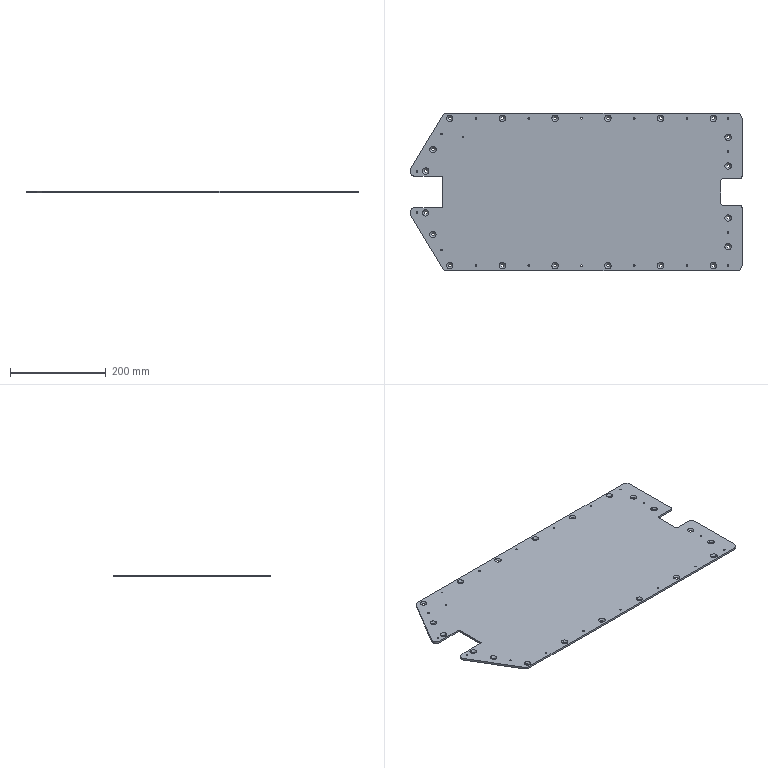Part | SolidWorks | features BaseBody 1 | 1 solid | 146 faces | box 692.069 x 328 x 4 mm | volume 839775 mm3 | cylinder 90 | cone 42 | plane 14 | commonest cylinder face diameters 6.2 x36 3.3 x32 20 x8 3.2 x4 6.4 x4 10 x4